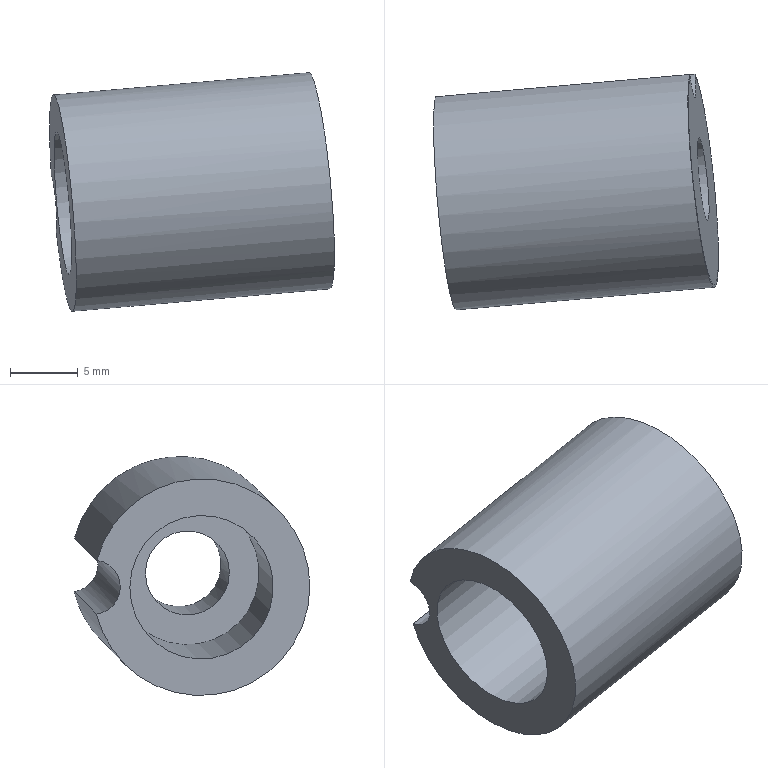Part | NX | features solid 2 | 1 solid | 8 faces | box 20.964 x 17.346 x 17.585 mm | volume 2437 mm3 | cylinder 4 | plane 2 | spline 2 | commonest cylinder face diameters 4 x1 6.2 x1 10.6 x1 16 x1
STEP:
#1=CARTESIAN_POINT('',(888.839,-112.459,34.948));
#2=VERTEX_POINT('',#1);
#3=CARTESIAN_POINT('',(870.12,-114.097,33.304));
#4=VERTEX_POINT('',#3);
#5=CARTESIAN_POINT('',(880.044,-113.228,34.176));
#6=DIRECTION('',(0.9924,0.08682,0.08716));
#7=VECTOR('',#6,1000.);
#8=LINE('',#5,#7);
#9=EDGE_CURVE('',#2,#4,#8,.F.);
#10=ORIENTED_EDGE('',*,*,#9,.T.);
#11=CARTESIAN_POINT('',(870.464,-114.067,29.351));
#12=VERTEX_POINT('',#11);
#13=CARTESIAN_POINT('',(870.967,-121.802,31.328));
#14=DIRECTION('',(-0.9924,-0.08682,-0.08716));
#15=DIRECTION('',(-0.08716,0.9962,0.));
#16=AXIS2_PLACEMENT_3D('',#13,#14,#15);
#17=CIRCLE('',#16,8.);
#18=EDGE_CURVE('',#12,#4,#17,.T.);
#19=ORIENTED_EDGE('',*,*,#18,.F.);
#20=CARTESIAN_POINT('',(889.222,-112.425,30.998));
#21=VERTEX_POINT('',#20);
#22=CARTESIAN_POINT('',(880.388,-113.198,30.222));
#23=DIRECTION('',(0.9924,0.08682,0.08716));
#24=VECTOR('',#23,1000.);
#25=LINE('',#22,#24);
#26=EDGE_CURVE('',#12,#21,#25,.T.);
#27=ORIENTED_EDGE('',*,*,#26,.T.);
#28=CARTESIAN_POINT('',(888.839,-112.459,34.948));
#29=CARTESIAN_POINT('',(888.707,-112.955,36.825));
#30=CARTESIAN_POINT('',(888.626,-115.329,40.152));
#31=CARTESIAN_POINT('',(889.1,-121.314,41.605));
#32=CARTESIAN_POINT('',(889.936,-126.712,38.737));
#33=CARTESIAN_POINT('',(890.715,-128.835,32.998));
#34=CARTESIAN_POINT('',(891.049,-126.618,27.251));
#35=CARTESIAN_POINT('',(890.77,-121.17,24.364));
#36=CARTESIAN_POINT('',(890.016,-115.208,25.802));
#37=CARTESIAN_POINT('',(889.453,-112.89,29.123));
#38=CARTESIAN_POINT('',(889.222,-112.425,30.998));
#39=B_SPLINE_CURVE_WITH_KNOTS('',3,(#28,#29,#30,#31,#32,#33,#34,#35,#36,#37,#38),.UNSPECIFIED.,.F.,.F.,(4,1,1,1,1,1,1,1,4),(0.,0.005755,0.01151,0.01726,0.02302,0.02877,0.03453,0.04028,0.04604),.UNSPECIFIED.);
#40=EDGE_CURVE('',#2,#21,#39,.T.);
#41=ORIENTED_EDGE('',*,*,#40,.F.);
#42=EDGE_LOOP('',(#10,#19,#27,#41));
#43=FACE_BOUND('',#42,.T.);
#44=CARTESIAN_POINT('',(870.967,-121.802,31.328));
#45=DIRECTION('',(0.9924,0.08682,0.08716));
#46=DIRECTION('',(-0.08716,0.9962,0.));
#47=AXIS2_PLACEMENT_3D('',#44,#45,#46);
#48=CYLINDRICAL_SURFACE('',#47,8.);
#49=ADVANCED_FACE('',(#43),#48,.T.);
#50=CARTESIAN_POINT('',(888.859,-112.623,34.921));
#51=VERTEX_POINT('',#50);
#52=CARTESIAN_POINT('',(888.839,-112.459,34.948));
#53=CARTESIAN_POINT('',(888.846,-112.514,34.941));
#54=CARTESIAN_POINT('',(888.852,-112.569,34.932));
#55=CARTESIAN_POINT('',(888.859,-112.623,34.921));
#56=B_SPLINE_CURVE_WITH_KNOTS('',3,(#52,#53,#54,#55),.UNSPECIFIED.,.F.,.F.,(4,4),(0.,0.0001659),.UNSPECIFIED.);
#57=EDGE_CURVE('',#2,#51,#56,.T.);
#58=ORIENTED_EDGE('',*,*,#57,.T.);
#59=CARTESIAN_POINT('',(889.236,-112.589,31.026));
#60=VERTEX_POINT('',#59);
#61=CARTESIAN_POINT('',(888.859,-112.623,34.921));
#62=CARTESIAN_POINT('',(888.968,-113.504,34.735));
#63=CARTESIAN_POINT('',(889.281,-114.875,32.977));
#64=CARTESIAN_POINT('',(889.309,-113.479,31.215));
#65=CARTESIAN_POINT('',(889.236,-112.589,31.026));
#66=B_SPLINE_CURVE_WITH_KNOTS('',3,(#61,#62,#63,#64,#65),.UNSPECIFIED.,.F.,.F.,(4,1,4),(0.0001659,0.002877,0.005588),.UNSPECIFIED.);
#67=EDGE_CURVE('',#51,#60,#66,.T.);
#68=ORIENTED_EDGE('',*,*,#67,.T.);
#69=CARTESIAN_POINT('',(889.236,-112.589,31.026));
#70=CARTESIAN_POINT('',(889.232,-112.535,31.014));
#71=CARTESIAN_POINT('',(889.227,-112.481,31.005));
#72=CARTESIAN_POINT('',(889.222,-112.425,30.998));
#73=B_SPLINE_CURVE_WITH_KNOTS('',3,(#69,#70,#71,#72),.UNSPECIFIED.,.F.,.F.,(4,4),(0.005588,0.005752),.UNSPECIFIED.);
#74=EDGE_CURVE('',#60,#21,#73,.T.);
#75=ORIENTED_EDGE('',*,*,#74,.T.);
#76=ORIENTED_EDGE('',*,*,#26,.F.);
#77=CARTESIAN_POINT('',(870.27,-113.833,31.328));
#78=DIRECTION('',(-0.9924,-0.08682,-0.08716));
#79=DIRECTION('',(-0.08716,0.9962,0.));
#80=AXIS2_PLACEMENT_3D('',#77,#78,#79);
#81=CIRCLE('',#80,2.);
#82=EDGE_CURVE('',#12,#4,#81,.T.);
#83=ORIENTED_EDGE('',*,*,#82,.T.);
#84=ORIENTED_EDGE('',*,*,#9,.F.);
#85=EDGE_LOOP('',(#58,#68,#75,#76,#83,#84));
#86=FACE_BOUND('',#85,.T.);
#87=CARTESIAN_POINT('',(870.27,-113.833,31.328));
#88=DIRECTION('',(0.9924,0.08682,0.08716));
#89=DIRECTION('',(-0.08716,0.9962,0.));
#90=AXIS2_PLACEMENT_3D('',#87,#88,#89);
#91=CYLINDRICAL_SURFACE('',#90,2.);
#92=ADVANCED_FACE('',(#86),#91,.F.);
#93=CARTESIAN_POINT('',(882.606,-117.672,32.373));
#94=VERTEX_POINT('',#93);
#95=CARTESIAN_POINT('',(882.876,-120.76,32.373));
#96=DIRECTION('',(-0.9924,-0.08682,-0.08716));
#97=DIRECTION('',(-0.08716,0.9962,0.));
#98=AXIS2_PLACEMENT_3D('',#95,#96,#97);
#99=CIRCLE('',#98,3.1);
#100=EDGE_CURVE('',#94,#94,#99,.T.);
#101=ORIENTED_EDGE('',*,*,#100,.T.);
#102=EDGE_LOOP('',(#101));
#103=FACE_BOUND('',#102,.T.);
#104=CARTESIAN_POINT('',(889.506,-117.068,32.979));
#105=VERTEX_POINT('',#104);
#106=CARTESIAN_POINT('',(889.809,-117.717,30.56));
#107=CARTESIAN_POINT('',(889.472,-116.734,32.979));
#108=CARTESIAN_POINT('',(889.34,-117.757,35.399));
#109=CARTESIAN_POINT('',(889.492,-120.179,36.402));
#110=CARTESIAN_POINT('',(889.837,-122.589,35.406));
#111=CARTESIAN_POINT('',(890.174,-123.57,32.989));
#112=CARTESIAN_POINT('',(890.306,-122.551,30.572));
#113=CARTESIAN_POINT('',(890.155,-120.127,29.564));
#114=CARTESIAN_POINT('',(889.809,-117.717,30.56));
#115=CARTESIAN_POINT('',(889.472,-116.734,32.979));
#116=CARTESIAN_POINT('',(889.34,-117.757,35.399));
#117=B_SPLINE_CURVE_WITH_KNOTS('',3,(#106,#107,#108,#109,#110,#111,#112,#113,#114,#115,#116),.UNSPECIFIED.,.T.,.F.,(1,1,1,1,1,1,1,1,1,1,1,1,1,1,1),(-0.007269,-0.004846,-0.002423,0.,0.002423,0.004846,0.007269,0.009692,0.01211,0.01454,0.01696,0.01938,0.02181,0.02423,0.02665),.UNSPECIFIED.);
#118=EDGE_CURVE('',#105,#105,#117,.T.);
#119=ORIENTED_EDGE('',*,*,#118,.T.);
#120=EDGE_LOOP('',(#119));
#121=FACE_BOUND('',#120,.T.);
#122=CARTESIAN_POINT('',(870.967,-121.802,31.328));
#123=DIRECTION('',(0.9924,0.08682,0.08716));
#124=DIRECTION('',(-0.08716,0.9962,0.));
#125=AXIS2_PLACEMENT_3D('',#122,#123,#124);
#126=CYLINDRICAL_SURFACE('',#125,3.1);
#127=ADVANCED_FACE('',(#103,#121),#126,.F.);
#128=CARTESIAN_POINT('',(870.505,-116.522,31.328));
#129=VERTEX_POINT('',#128);
#130=CARTESIAN_POINT('',(870.967,-121.802,31.328));
#131=DIRECTION('',(-0.9924,-0.08682,-0.08716));
#132=DIRECTION('',(-0.08716,0.9962,0.));
#133=AXIS2_PLACEMENT_3D('',#130,#131,#132);
#134=CIRCLE('',#133,5.3);
#135=EDGE_CURVE('',#129,#129,#134,.T.);
#136=ORIENTED_EDGE('',*,*,#135,.F.);
#137=EDGE_LOOP('',(#136));
#138=FACE_BOUND('',#137,.T.);
#139=ORIENTED_EDGE('',*,*,#18,.T.);
#140=ORIENTED_EDGE('',*,*,#82,.F.);
#141=EDGE_LOOP('',(#139,#140));
#142=FACE_BOUND('',#141,.T.);
#143=CARTESIAN_POINT('',(870.967,-121.802,31.328));
#144=DIRECTION('',(0.9924,0.08682,0.08716));
#145=DIRECTION('',(-0.08716,0.9962,0.));
#146=AXIS2_PLACEMENT_3D('',#143,#144,#145);
#147=PLANE('',#146);
#148=ADVANCED_FACE('',(#138,#142),#147,.F.);
#149=ORIENTED_EDGE('',*,*,#135,.T.);
#150=EDGE_LOOP('',(#149));
#151=FACE_BOUND('',#150,.T.);
#152=CARTESIAN_POINT('',(882.414,-115.48,32.373));
#153=VERTEX_POINT('',#152);
#154=CARTESIAN_POINT('',(882.876,-120.76,32.373));
#155=DIRECTION('',(-0.9924,-0.08682,-0.08716));
#156=DIRECTION('',(-0.08716,0.9962,0.));
#157=AXIS2_PLACEMENT_3D('',#154,#155,#156);
#158=CIRCLE('',#157,5.3);
#159=EDGE_CURVE('',#153,#153,#158,.T.);
#160=ORIENTED_EDGE('',*,*,#159,.F.);
#161=EDGE_LOOP('',(#160));
#162=FACE_BOUND('',#161,.T.);
#163=CARTESIAN_POINT('',(870.967,-121.802,31.328));
#164=DIRECTION('',(0.9924,0.08682,0.08716));
#165=DIRECTION('',(-0.08716,0.9962,0.));
#166=AXIS2_PLACEMENT_3D('',#163,#164,#165);
#167=CYLINDRICAL_SURFACE('',#166,5.3);
#168=ADVANCED_FACE('',(#151,#162),#167,.F.);
#169=ORIENTED_EDGE('',*,*,#100,.F.);
#170=EDGE_LOOP('',(#169));
#171=FACE_BOUND('',#170,.T.);
#172=ORIENTED_EDGE('',*,*,#159,.T.);
#173=EDGE_LOOP('',(#172));
#174=FACE_BOUND('',#173,.T.);
#175=CARTESIAN_POINT('',(882.876,-120.76,32.373));
#176=DIRECTION('',(0.9924,0.08682,0.08716));
#177=DIRECTION('',(-0.08716,0.9962,0.));
#178=AXIS2_PLACEMENT_3D('',#175,#176,#177);
#179=PLANE('',#178);
#180=ADVANCED_FACE('',(#171,#174),#179,.F.);
#181=ORIENTED_EDGE('',*,*,#40,.T.);
#182=ORIENTED_EDGE('',*,*,#74,.F.);
#183=CARTESIAN_POINT('',(890.576,-120.072,25.191));
#184=VERTEX_POINT('',#183);
#185=CARTESIAN_POINT('',(890.576,-120.072,25.191));
#186=CARTESIAN_POINT('',(890.398,-118.34,25.191));
#187=CARTESIAN_POINT('',(889.939,-114.979,26.347));
#188=CARTESIAN_POINT('',(889.439,-113.001,29.38));
#189=CARTESIAN_POINT('',(889.236,-112.589,31.026));
#190=B_SPLINE_CURVE_WITH_KNOTS('',3,(#185,#186,#187,#188,#189),.UNSPECIFIED.,.F.,.F.,(4,1,4),(0.,0.2093,0.4187),.UNSPECIFIED.);
#191=EDGE_CURVE('',#184,#60,#190,.T.);
#192=ORIENTED_EDGE('',*,*,#191,.F.);
#193=CARTESIAN_POINT('',(889.069,-120.223,40.775));
#194=VERTEX_POINT('',#193);
#195=CARTESIAN_POINT('',(889.069,-120.223,40.775));
#196=CARTESIAN_POINT('',(889.281,-122.289,40.775));
#197=CARTESIAN_POINT('',(889.858,-126.293,39.09));
#198=CARTESIAN_POINT('',(890.711,-128.786,32.985));
#199=CARTESIAN_POINT('',(891.04,-126.174,26.879));
#200=CARTESIAN_POINT('',(890.789,-122.139,25.192));
#201=CARTESIAN_POINT('',(890.576,-120.072,25.191));
#202=B_SPLINE_CURVE_WITH_KNOTS('',3,(#195,#196,#197,#198,#199,#200,#201),.UNSPECIFIED.,.F.,.F.,(4,1,1,1,4),(0.,0.25,0.5,0.75,1.),.UNSPECIFIED.);
#203=EDGE_CURVE('',#194,#184,#202,.T.);
#204=ORIENTED_EDGE('',*,*,#203,.F.);
#205=CARTESIAN_POINT('',(888.859,-112.623,34.921));
#206=CARTESIAN_POINT('',(888.743,-113.064,36.57));
#207=CARTESIAN_POINT('',(888.655,-115.094,39.608));
#208=CARTESIAN_POINT('',(888.89,-118.485,40.774));
#209=CARTESIAN_POINT('',(889.069,-120.223,40.775));
#210=B_SPLINE_CURVE_WITH_KNOTS('',3,(#205,#206,#207,#208,#209),.UNSPECIFIED.,.F.,.F.,(4,1,4),(0.5798,0.7899,1.),.UNSPECIFIED.);
#211=EDGE_CURVE('',#51,#194,#210,.T.);
#212=ORIENTED_EDGE('',*,*,#211,.F.);
#213=ORIENTED_EDGE('',*,*,#57,.F.);
#214=EDGE_LOOP('',(#181,#182,#192,#204,#212,#213));
#215=FACE_BOUND('',#214,.T.);
#216=CARTESIAN_POINT('',(889.875,-128.329,41.066));
#217=CARTESIAN_POINT('',(891.44,-128.173,24.882));
#218=CARTESIAN_POINT('',(888.238,-112.424,41.062));
#219=CARTESIAN_POINT('',(889.804,-112.267,24.878));
#220=B_SPLINE_SURFACE_WITH_KNOTS('',1,1,((#216,#217),(#218,#219)),.PLANE_SURF.,.F.,.F.,.F.,(2,2),(2,2),(0.658,0.7769),(0.1984,0.4556),.PIECEWISE_BEZIER_KNOTS.);
#221=ADVANCED_FACE('',(#215),#220,.F.);
#222=ORIENTED_EDGE('',*,*,#118,.F.);
#223=EDGE_LOOP('',(#222));
#224=FACE_BOUND('',#223,.T.);
#225=ORIENTED_EDGE('',*,*,#211,.T.);
#226=ORIENTED_EDGE('',*,*,#203,.T.);
#227=ORIENTED_EDGE('',*,*,#191,.T.);
#228=ORIENTED_EDGE('',*,*,#67,.F.);
#229=EDGE_LOOP('',(#225,#226,#227,#228));
#230=FACE_BOUND('',#229,.T.);
#231=CARTESIAN_POINT('',(889.87,-128.103,40.87));
#232=CARTESIAN_POINT('',(891.396,-127.95,25.1));
#233=CARTESIAN_POINT('',(888.274,-112.588,40.866));
#234=CARTESIAN_POINT('',(889.8,-112.436,25.096));
#235=B_SPLINE_SURFACE_WITH_KNOTS('',1,1,((#231,#232),(#233,#234)),.PLANE_SURF.,.F.,.F.,.F.,(2,2),(2,2),(0.6596,0.7757),(0.2016,0.4521),.PIECEWISE_BEZIER_KNOTS.);
#236=ADVANCED_FACE('',(#224,#230),#235,.F.);
#237=CLOSED_SHELL('',(#49,#92,#127,#148,#168,#180,#221,#236));
#238=MANIFOLD_SOLID_BREP('',#237);
#239=(LENGTH_UNIT()NAMED_UNIT(*)SI_UNIT(.MILLI.,.METRE.));
#240=UNCERTAINTY_MEASURE_WITH_UNIT(LENGTH_MEASURE(0.0508),#239,'','');
#241=(NAMED_UNIT(*)PLANE_ANGLE_UNIT()SI_UNIT($,.RADIAN.));
#242=(NAMED_UNIT(*)SI_UNIT($,.STERADIAN.)SOLID_ANGLE_UNIT());
#243=(GEOMETRIC_REPRESENTATION_CONTEXT(3)GLOBAL_UNCERTAINTY_ASSIGNED_CONTEXT((#240))GLOBAL_UNIT_ASSIGNED_CONTEXT((#239,#241,#242))REPRESENTATION_CONTEXT('',''));
#244=ADVANCED_BREP_SHAPE_REPRESENTATION('',(#238),#243);